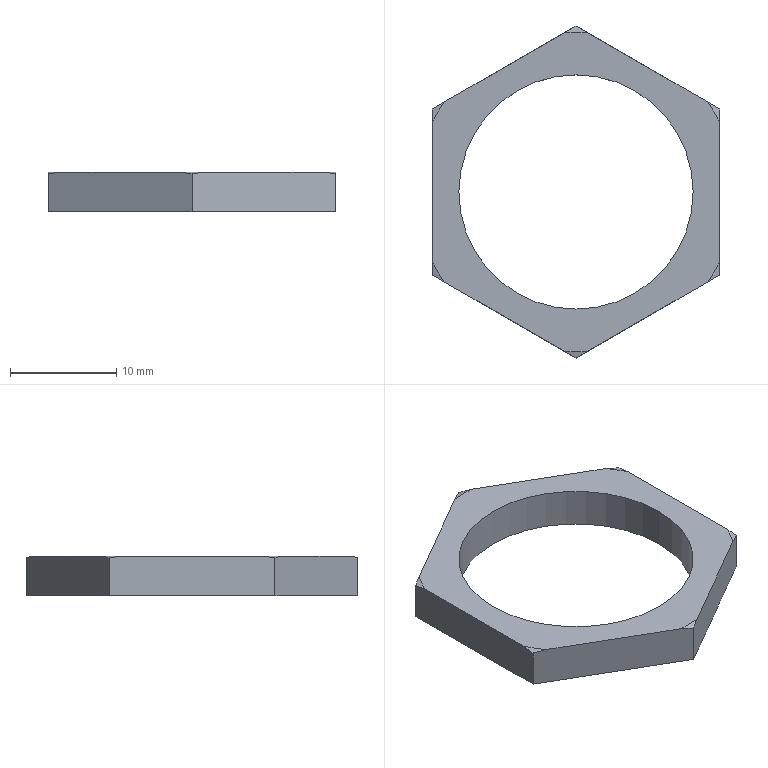Part | STEP file | PN_0023[ PN_0023]_GB/T 808-1988 small hex thin nut M22×1(A3)_Nut M22×1 | 1 solid | 16 faces | box 27 x 31.177 x 3.74 mm | volume 939.292 mm3 | plane 8 | cone 6 | cylinder 2 | commonest cylinder face diameters 22 x2
STEP:
#1=CARTESIAN_POINT('',(-11.,0.,3.74));
#2=VERTEX_POINT('',#1);
#3=CARTESIAN_POINT('',(11.,0.,3.74));
#4=VERTEX_POINT('',#3);
#5=CARTESIAN_POINT('',(0.,0.,3.74));
#6=DIRECTION('',(0.,0.,1.));
#7=DIRECTION('',(1.,0.,0.));
#8=AXIS2_PLACEMENT_3D('',#5,#6,#7);
#9=CIRCLE('',#8,11.);
#10=EDGE_CURVE('',#2,#4,#9,.T.);
#11=ORIENTED_EDGE('',*,*,#10,.T.);
#12=CARTESIAN_POINT('',(11.,0.,0.));
#13=VERTEX_POINT('',#12);
#14=CARTESIAN_POINT('',(11.,0.,3.74));
#15=DIRECTION('',(0.,0.,-1.));
#16=VECTOR('',#15,1000.);
#17=LINE('',#14,#16);
#18=EDGE_CURVE('',#4,#13,#17,.T.);
#19=ORIENTED_EDGE('',*,*,#18,.T.);
#20=CARTESIAN_POINT('',(-11.,0.,0.));
#21=VERTEX_POINT('',#20);
#22=CARTESIAN_POINT('',(0.,0.,0.));
#23=DIRECTION('',(0.,0.,1.));
#24=DIRECTION('',(1.,0.,0.));
#25=AXIS2_PLACEMENT_3D('',#22,#23,#24);
#26=CIRCLE('',#25,11.);
#27=EDGE_CURVE('',#21,#13,#26,.T.);
#28=ORIENTED_EDGE('',*,*,#27,.F.);
#29=CARTESIAN_POINT('',(-11.,0.,3.74));
#30=DIRECTION('',(0.,0.,-1.));
#31=VECTOR('',#30,1000.);
#32=LINE('',#29,#31);
#33=EDGE_CURVE('',#2,#21,#32,.T.);
#34=ORIENTED_EDGE('',*,*,#33,.F.);
#35=EDGE_LOOP('',(#11,#19,#28,#34));
#36=FACE_OUTER_BOUND('',#35,.T.);
#37=CARTESIAN_POINT('',(0.,0.,3.74));
#38=DIRECTION('',(0.,0.,-1.));
#39=DIRECTION('',(-1.,0.,0.));
#40=AXIS2_PLACEMENT_3D('',#37,#38,#39);
#41=CYLINDRICAL_SURFACE('',#40,11.);
#42=ADVANCED_FACE('',(#36),#41,.F.);
#43=ORIENTED_EDGE('',*,*,#10,.F.);
#44=CARTESIAN_POINT('',(0.,0.,3.74));
#45=DIRECTION('',(0.,0.,1.));
#46=DIRECTION('',(1.,0.,0.));
#47=AXIS2_PLACEMENT_3D('',#44,#45,#46);
#48=CIRCLE('',#47,11.);
#49=EDGE_CURVE('',#4,#2,#48,.T.);
#50=ORIENTED_EDGE('',*,*,#49,.F.);
#51=EDGE_LOOP('',(#43,#50));
#52=FACE_BOUND('',#51,.T.);
#53=CARTESIAN_POINT('',(-12.412,8.422,3.74));
#54=VERTEX_POINT('',#53);
#55=CARTESIAN_POINT('',(-13.5,6.538,3.74));
#56=VERTEX_POINT('',#55);
#57=CARTESIAN_POINT('',(0.,0.,3.74));
#58=DIRECTION('',(0.,0.,1.));
#59=DIRECTION('',(1.,0.,0.));
#60=AXIS2_PLACEMENT_3D('',#57,#58,#59);
#61=CIRCLE('',#60,15.);
#62=EDGE_CURVE('',#54,#56,#61,.T.);
#63=ORIENTED_EDGE('',*,*,#62,.T.);
#64=CARTESIAN_POINT('',(-13.5,-6.538,3.74));
#65=VERTEX_POINT('',#64);
#66=CARTESIAN_POINT('',(-13.5,7.794,3.74));
#67=DIRECTION('',(0.,-1.,0.));
#68=VECTOR('',#67,1000.);
#69=LINE('',#66,#68);
#70=EDGE_CURVE('',#56,#65,#69,.T.);
#71=ORIENTED_EDGE('',*,*,#70,.T.);
#72=CARTESIAN_POINT('',(-12.412,-8.422,3.74));
#73=VERTEX_POINT('',#72);
#74=CARTESIAN_POINT('',(0.,0.,3.74));
#75=DIRECTION('',(0.,0.,1.));
#76=DIRECTION('',(1.,0.,0.));
#77=AXIS2_PLACEMENT_3D('',#74,#75,#76);
#78=CIRCLE('',#77,15.);
#79=EDGE_CURVE('',#65,#73,#78,.T.);
#80=ORIENTED_EDGE('',*,*,#79,.T.);
#81=CARTESIAN_POINT('',(-1.088,-14.961,3.74));
#82=VERTEX_POINT('',#81);
#83=CARTESIAN_POINT('',(-13.5,-7.794,3.74));
#84=DIRECTION('',(0.866,-0.5,0.));
#85=VECTOR('',#84,1000.);
#86=LINE('',#83,#85);
#87=EDGE_CURVE('',#73,#82,#86,.T.);
#88=ORIENTED_EDGE('',*,*,#87,.T.);
#89=CARTESIAN_POINT('',(1.088,-14.961,3.74));
#90=VERTEX_POINT('',#89);
#91=CARTESIAN_POINT('',(0.,0.,3.74));
#92=DIRECTION('',(0.,0.,1.));
#93=DIRECTION('',(1.,0.,0.));
#94=AXIS2_PLACEMENT_3D('',#91,#92,#93);
#95=CIRCLE('',#94,15.);
#96=EDGE_CURVE('',#82,#90,#95,.T.);
#97=ORIENTED_EDGE('',*,*,#96,.T.);
#98=CARTESIAN_POINT('',(12.412,-8.422,3.74));
#99=VERTEX_POINT('',#98);
#100=CARTESIAN_POINT('',(0.,-15.588,3.74));
#101=DIRECTION('',(0.866,0.5,0.));
#102=VECTOR('',#101,1000.);
#103=LINE('',#100,#102);
#104=EDGE_CURVE('',#90,#99,#103,.T.);
#105=ORIENTED_EDGE('',*,*,#104,.T.);
#106=CARTESIAN_POINT('',(13.5,-6.538,3.74));
#107=VERTEX_POINT('',#106);
#108=CARTESIAN_POINT('',(0.,0.,3.74));
#109=DIRECTION('',(0.,0.,1.));
#110=DIRECTION('',(1.,0.,0.));
#111=AXIS2_PLACEMENT_3D('',#108,#109,#110);
#112=CIRCLE('',#111,15.);
#113=EDGE_CURVE('',#99,#107,#112,.T.);
#114=ORIENTED_EDGE('',*,*,#113,.T.);
#115=CARTESIAN_POINT('',(13.5,6.538,3.74));
#116=VERTEX_POINT('',#115);
#117=CARTESIAN_POINT('',(13.5,-7.794,3.74));
#118=DIRECTION('',(0.,1.,0.));
#119=VECTOR('',#118,1000.);
#120=LINE('',#117,#119);
#121=EDGE_CURVE('',#107,#116,#120,.T.);
#122=ORIENTED_EDGE('',*,*,#121,.T.);
#123=CARTESIAN_POINT('',(12.412,8.422,3.74));
#124=VERTEX_POINT('',#123);
#125=CARTESIAN_POINT('',(0.,0.,3.74));
#126=DIRECTION('',(0.,0.,1.));
#127=DIRECTION('',(1.,0.,0.));
#128=AXIS2_PLACEMENT_3D('',#125,#126,#127);
#129=CIRCLE('',#128,15.);
#130=EDGE_CURVE('',#116,#124,#129,.T.);
#131=ORIENTED_EDGE('',*,*,#130,.T.);
#132=CARTESIAN_POINT('',(1.088,14.961,3.74));
#133=VERTEX_POINT('',#132);
#134=CARTESIAN_POINT('',(13.5,7.794,3.74));
#135=DIRECTION('',(-0.866,0.5,0.));
#136=VECTOR('',#135,1000.);
#137=LINE('',#134,#136);
#138=EDGE_CURVE('',#124,#133,#137,.T.);
#139=ORIENTED_EDGE('',*,*,#138,.T.);
#140=CARTESIAN_POINT('',(-1.088,14.961,3.74));
#141=VERTEX_POINT('',#140);
#142=CARTESIAN_POINT('',(0.,0.,3.74));
#143=DIRECTION('',(0.,0.,1.));
#144=DIRECTION('',(1.,0.,0.));
#145=AXIS2_PLACEMENT_3D('',#142,#143,#144);
#146=CIRCLE('',#145,15.);
#147=EDGE_CURVE('',#133,#141,#146,.T.);
#148=ORIENTED_EDGE('',*,*,#147,.T.);
#149=CARTESIAN_POINT('',(0.,15.588,3.74));
#150=DIRECTION('',(-0.866,-0.5,0.));
#151=VECTOR('',#150,1000.);
#152=LINE('',#149,#151);
#153=EDGE_CURVE('',#141,#54,#152,.T.);
#154=ORIENTED_EDGE('',*,*,#153,.T.);
#155=EDGE_LOOP('',(#63,#71,#80,#88,#97,#105,#114,#122,#131,#139,#148,#154));
#156=FACE_OUTER_BOUND('',#155,.T.);
#157=CARTESIAN_POINT('',(27.,0.,3.74));
#158=DIRECTION('',(0.,0.,-1.));
#159=DIRECTION('',(-1.,0.,0.));
#160=AXIS2_PLACEMENT_3D('',#157,#158,#159);
#161=PLANE('',#160);
#162=ADVANCED_FACE('',(#52,#156),#161,.F.);
#163=CARTESIAN_POINT('',(13.5,7.794,3.582));
#164=VERTEX_POINT('',#163);
#165=CARTESIAN_POINT('',(13.5,7.794,3.582));
#166=CARTESIAN_POINT('',(13.138,8.003,3.638));
#167=CARTESIAN_POINT('',(12.775,8.213,3.691));
#168=CARTESIAN_POINT('',(12.412,8.422,3.74));
#169=B_SPLINE_CURVE_WITH_KNOTS('',3,(#165,#166,#167,#168),.UNSPECIFIED.,.F.,.F.,(4,4),(0.01126,0.01252),.UNSPECIFIED.);
#170=EDGE_CURVE('',#164,#124,#169,.T.);
#171=ORIENTED_EDGE('',*,*,#170,.F.);
#172=CARTESIAN_POINT('',(13.5,7.794,0.));
#173=VERTEX_POINT('',#172);
#174=CARTESIAN_POINT('',(13.5,7.794,3.74));
#175=DIRECTION('',(0.,0.,-1.));
#176=VECTOR('',#175,1000.);
#177=LINE('',#174,#176);
#178=EDGE_CURVE('',#164,#173,#177,.T.);
#179=ORIENTED_EDGE('',*,*,#178,.T.);
#180=CARTESIAN_POINT('',(0.,15.588,0.));
#181=VERTEX_POINT('',#180);
#182=CARTESIAN_POINT('',(13.5,7.794,0.));
#183=DIRECTION('',(-0.866,0.5,0.));
#184=VECTOR('',#183,1000.);
#185=LINE('',#182,#184);
#186=EDGE_CURVE('',#173,#181,#185,.T.);
#187=ORIENTED_EDGE('',*,*,#186,.T.);
#188=CARTESIAN_POINT('',(0.,15.588,3.582));
#189=VERTEX_POINT('',#188);
#190=CARTESIAN_POINT('',(0.,15.588,3.74));
#191=DIRECTION('',(0.,0.,-1.));
#192=VECTOR('',#191,1000.);
#193=LINE('',#190,#192);
#194=EDGE_CURVE('',#189,#181,#193,.T.);
#195=ORIENTED_EDGE('',*,*,#194,.F.);
#196=CARTESIAN_POINT('',(1.088,14.961,3.74));
#197=CARTESIAN_POINT('',(0.7246,15.17,3.691));
#198=CARTESIAN_POINT('',(0.362,15.379,3.638));
#199=CARTESIAN_POINT('',(0.,15.588,3.582));
#200=B_SPLINE_CURVE_WITH_KNOTS('',3,(#196,#197,#198,#199),.UNSPECIFIED.,.F.,.F.,(4,4),(0.02554,0.02678),.UNSPECIFIED.);
#201=EDGE_CURVE('',#133,#189,#200,.T.);
#202=ORIENTED_EDGE('',*,*,#201,.F.);
#203=ORIENTED_EDGE('',*,*,#138,.F.);
#204=EDGE_LOOP('',(#171,#179,#187,#195,#202,#203));
#205=FACE_OUTER_BOUND('',#204,.T.);
#206=CARTESIAN_POINT('',(13.5,7.794,3.74));
#207=DIRECTION('',(-0.5,-0.866,0.));
#208=DIRECTION('',(0.866,-0.5,0.));
#209=AXIS2_PLACEMENT_3D('',#206,#207,#208);
#210=PLANE('',#209);
#211=ADVANCED_FACE('',(#205),#210,.F.);
#212=CARTESIAN_POINT('',(0.,15.588,3.582));
#213=CARTESIAN_POINT('',(-0.3622,15.379,3.638));
#214=CARTESIAN_POINT('',(-0.7248,15.17,3.691));
#215=CARTESIAN_POINT('',(-1.088,14.961,3.74));
#216=B_SPLINE_CURVE_WITH_KNOTS('',3,(#212,#213,#214,#215),.UNSPECIFIED.,.F.,.F.,(4,4),(0.01126,0.01252),.UNSPECIFIED.);
#217=EDGE_CURVE('',#189,#141,#216,.T.);
#218=ORIENTED_EDGE('',*,*,#217,.F.);
#219=ORIENTED_EDGE('',*,*,#194,.T.);
#220=CARTESIAN_POINT('',(-13.5,7.794,0.));
#221=VERTEX_POINT('',#220);
#222=CARTESIAN_POINT('',(0.,15.588,0.));
#223=DIRECTION('',(-0.866,-0.5,0.));
#224=VECTOR('',#223,1000.);
#225=LINE('',#222,#224);
#226=EDGE_CURVE('',#181,#221,#225,.T.);
#227=ORIENTED_EDGE('',*,*,#226,.T.);
#228=CARTESIAN_POINT('',(-13.5,7.794,3.582));
#229=VERTEX_POINT('',#228);
#230=CARTESIAN_POINT('',(-13.5,7.794,3.74));
#231=DIRECTION('',(0.,0.,-1.));
#232=VECTOR('',#231,1000.);
#233=LINE('',#230,#232);
#234=EDGE_CURVE('',#229,#221,#233,.T.);
#235=ORIENTED_EDGE('',*,*,#234,.F.);
#236=CARTESIAN_POINT('',(-12.412,8.422,3.74));
#237=CARTESIAN_POINT('',(-12.775,8.213,3.691));
#238=CARTESIAN_POINT('',(-13.138,8.003,3.638));
#239=CARTESIAN_POINT('',(-13.5,7.794,3.582));
#240=B_SPLINE_CURVE_WITH_KNOTS('',3,(#236,#237,#238,#239),.UNSPECIFIED.,.F.,.F.,(4,4),(0.02554,0.02678),.UNSPECIFIED.);
#241=EDGE_CURVE('',#54,#229,#240,.T.);
#242=ORIENTED_EDGE('',*,*,#241,.F.);
#243=ORIENTED_EDGE('',*,*,#153,.F.);
#244=EDGE_LOOP('',(#218,#219,#227,#235,#242,#243));
#245=FACE_OUTER_BOUND('',#244,.T.);
#246=CARTESIAN_POINT('',(0.,15.588,3.74));
#247=DIRECTION('',(0.5,-0.866,0.));
#248=DIRECTION('',(0.866,0.5,0.));
#249=AXIS2_PLACEMENT_3D('',#246,#247,#248);
#250=PLANE('',#249);
#251=ADVANCED_FACE('',(#245),#250,.F.);
#252=CARTESIAN_POINT('',(-13.5,7.794,3.582));
#253=CARTESIAN_POINT('',(-13.5,7.376,3.638));
#254=CARTESIAN_POINT('',(-13.5,6.957,3.691));
#255=CARTESIAN_POINT('',(-13.5,6.538,3.74));
#256=B_SPLINE_CURVE_WITH_KNOTS('',3,(#252,#253,#254,#255),.UNSPECIFIED.,.F.,.F.,(4,4),(0.009735,0.011),.UNSPECIFIED.);
#257=EDGE_CURVE('',#229,#56,#256,.T.);
#258=ORIENTED_EDGE('',*,*,#257,.F.);
#259=ORIENTED_EDGE('',*,*,#234,.T.);
#260=CARTESIAN_POINT('',(-13.5,-7.794,0.));
#261=VERTEX_POINT('',#260);
#262=CARTESIAN_POINT('',(-13.5,7.794,0.));
#263=DIRECTION('',(0.,-1.,0.));
#264=VECTOR('',#263,1000.);
#265=LINE('',#262,#264);
#266=EDGE_CURVE('',#221,#261,#265,.T.);
#267=ORIENTED_EDGE('',*,*,#266,.T.);
#268=CARTESIAN_POINT('',(-13.5,-7.794,3.582));
#269=VERTEX_POINT('',#268);
#270=CARTESIAN_POINT('',(-13.5,-7.794,3.74));
#271=DIRECTION('',(0.,0.,-1.));
#272=VECTOR('',#271,1000.);
#273=LINE('',#270,#272);
#274=EDGE_CURVE('',#269,#261,#273,.T.);
#275=ORIENTED_EDGE('',*,*,#274,.F.);
#276=CARTESIAN_POINT('',(-13.5,-6.538,3.74));
#277=CARTESIAN_POINT('',(-13.5,-6.958,3.691));
#278=CARTESIAN_POINT('',(-13.5,-7.376,3.638));
#279=CARTESIAN_POINT('',(-13.5,-7.794,3.582));
#280=B_SPLINE_CURVE_WITH_KNOTS('',3,(#276,#277,#278,#279),.UNSPECIFIED.,.F.,.F.,(4,4),(0.02403,0.02527),.UNSPECIFIED.);
#281=EDGE_CURVE('',#65,#269,#280,.T.);
#282=ORIENTED_EDGE('',*,*,#281,.F.);
#283=ORIENTED_EDGE('',*,*,#70,.F.);
#284=EDGE_LOOP('',(#258,#259,#267,#275,#282,#283));
#285=FACE_OUTER_BOUND('',#284,.T.);
#286=CARTESIAN_POINT('',(-13.5,7.794,3.74));
#287=DIRECTION('',(1.,0.,0.));
#288=DIRECTION('',(0.,1.,0.));
#289=AXIS2_PLACEMENT_3D('',#286,#287,#288);
#290=PLANE('',#289);
#291=ADVANCED_FACE('',(#285),#290,.F.);
#292=CARTESIAN_POINT('',(-13.5,-7.794,3.582));
#293=CARTESIAN_POINT('',(-13.138,-8.003,3.638));
#294=CARTESIAN_POINT('',(-12.775,-8.213,3.691));
#295=CARTESIAN_POINT('',(-12.412,-8.422,3.74));
#296=B_SPLINE_CURVE_WITH_KNOTS('',3,(#292,#293,#294,#295),.UNSPECIFIED.,.F.,.F.,(4,4),(0.01126,0.01252),.UNSPECIFIED.);
#297=EDGE_CURVE('',#269,#73,#296,.T.);
#298=ORIENTED_EDGE('',*,*,#297,.F.);
#299=ORIENTED_EDGE('',*,*,#274,.T.);
#300=CARTESIAN_POINT('',(0.,-15.588,0.));
#301=VERTEX_POINT('',#300);
#302=CARTESIAN_POINT('',(-13.5,-7.794,0.));
#303=DIRECTION('',(0.866,-0.5,0.));
#304=VECTOR('',#303,1000.);
#305=LINE('',#302,#304);
#306=EDGE_CURVE('',#261,#301,#305,.T.);
#307=ORIENTED_EDGE('',*,*,#306,.T.);
#308=CARTESIAN_POINT('',(0.,-15.588,3.582));
#309=VERTEX_POINT('',#308);
#310=CARTESIAN_POINT('',(0.,-15.588,3.74));
#311=DIRECTION('',(0.,0.,-1.));
#312=VECTOR('',#311,1000.);
#313=LINE('',#310,#312);
#314=EDGE_CURVE('',#309,#301,#313,.T.);
#315=ORIENTED_EDGE('',*,*,#314,.F.);
#316=CARTESIAN_POINT('',(-1.088,-14.961,3.74));
#317=CARTESIAN_POINT('',(-0.7246,-15.17,3.691));
#318=CARTESIAN_POINT('',(-0.362,-15.379,3.638));
#319=CARTESIAN_POINT('',(0.,-15.588,3.582));
#320=B_SPLINE_CURVE_WITH_KNOTS('',3,(#316,#317,#318,#319),.UNSPECIFIED.,.F.,.F.,(4,4),(0.02554,0.02678),.UNSPECIFIED.);
#321=EDGE_CURVE('',#82,#309,#320,.T.);
#322=ORIENTED_EDGE('',*,*,#321,.F.);
#323=ORIENTED_EDGE('',*,*,#87,.F.);
#324=EDGE_LOOP('',(#298,#299,#307,#315,#322,#323));
#325=FACE_OUTER_BOUND('',#324,.T.);
#326=CARTESIAN_POINT('',(-13.5,-7.794,3.74));
#327=DIRECTION('',(0.5,0.866,0.));
#328=DIRECTION('',(-0.866,0.5,0.));
#329=AXIS2_PLACEMENT_3D('',#326,#327,#328);
#330=PLANE('',#329);
#331=ADVANCED_FACE('',(#325),#330,.F.);
#332=CARTESIAN_POINT('',(0.,-15.588,3.582));
#333=CARTESIAN_POINT('',(0.3622,-15.379,3.638));
#334=CARTESIAN_POINT('',(0.7248,-15.17,3.691));
#335=CARTESIAN_POINT('',(1.088,-14.961,3.74));
#336=B_SPLINE_CURVE_WITH_KNOTS('',3,(#332,#333,#334,#335),.UNSPECIFIED.,.F.,.F.,(4,4),(0.01126,0.01252),.UNSPECIFIED.);
#337=EDGE_CURVE('',#309,#90,#336,.T.);
#338=ORIENTED_EDGE('',*,*,#337,.F.);
#339=ORIENTED_EDGE('',*,*,#314,.T.);
#340=CARTESIAN_POINT('',(13.5,-7.794,0.));
#341=VERTEX_POINT('',#340);
#342=CARTESIAN_POINT('',(0.,-15.588,0.));
#343=DIRECTION('',(0.866,0.5,0.));
#344=VECTOR('',#343,1000.);
#345=LINE('',#342,#344);
#346=EDGE_CURVE('',#301,#341,#345,.T.);
#347=ORIENTED_EDGE('',*,*,#346,.T.);
#348=CARTESIAN_POINT('',(13.5,-7.794,3.582));
#349=VERTEX_POINT('',#348);
#350=CARTESIAN_POINT('',(13.5,-7.794,3.74));
#351=DIRECTION('',(0.,0.,-1.));
#352=VECTOR('',#351,1000.);
#353=LINE('',#350,#352);
#354=EDGE_CURVE('',#349,#341,#353,.T.);
#355=ORIENTED_EDGE('',*,*,#354,.F.);
#356=CARTESIAN_POINT('',(12.412,-8.422,3.74));
#357=CARTESIAN_POINT('',(12.775,-8.213,3.691));
#358=CARTESIAN_POINT('',(13.138,-8.003,3.638));
#359=CARTESIAN_POINT('',(13.5,-7.794,3.582));
#360=B_SPLINE_CURVE_WITH_KNOTS('',3,(#356,#357,#358,#359),.UNSPECIFIED.,.F.,.F.,(4,4),(0.02554,0.02678),.UNSPECIFIED.);
#361=EDGE_CURVE('',#99,#349,#360,.T.);
#362=ORIENTED_EDGE('',*,*,#361,.F.);
#363=ORIENTED_EDGE('',*,*,#104,.F.);
#364=EDGE_LOOP('',(#338,#339,#347,#355,#362,#363));
#365=FACE_OUTER_BOUND('',#364,.T.);
#366=CARTESIAN_POINT('',(0.,-15.588,3.74));
#367=DIRECTION('',(-0.5,0.866,0.));
#368=DIRECTION('',(-0.866,-0.5,0.));
#369=AXIS2_PLACEMENT_3D('',#366,#367,#368);
#370=PLANE('',#369);
#371=ADVANCED_FACE('',(#365),#370,.F.);
#372=CARTESIAN_POINT('',(13.5,-7.794,3.582));
#373=CARTESIAN_POINT('',(13.5,-7.376,3.638));
#374=CARTESIAN_POINT('',(13.5,-6.957,3.691));
#375=CARTESIAN_POINT('',(13.5,-6.538,3.74));
#376=B_SPLINE_CURVE_WITH_KNOTS('',3,(#372,#373,#374,#375),.UNSPECIFIED.,.F.,.F.,(4,4),(0.009735,0.011),.UNSPECIFIED.);
#377=EDGE_CURVE('',#349,#107,#376,.T.);
#378=ORIENTED_EDGE('',*,*,#377,.F.);
#379=ORIENTED_EDGE('',*,*,#354,.T.);
#380=CARTESIAN_POINT('',(13.5,-7.794,0.));
#381=DIRECTION('',(0.,1.,0.));
#382=VECTOR('',#381,1000.);
#383=LINE('',#380,#382);
#384=EDGE_CURVE('',#341,#173,#383,.T.);
#385=ORIENTED_EDGE('',*,*,#384,.T.);
#386=ORIENTED_EDGE('',*,*,#178,.F.);
#387=CARTESIAN_POINT('',(13.5,6.538,3.74));
#388=CARTESIAN_POINT('',(13.5,6.958,3.691));
#389=CARTESIAN_POINT('',(13.5,7.376,3.638));
#390=CARTESIAN_POINT('',(13.5,7.794,3.582));
#391=B_SPLINE_CURVE_WITH_KNOTS('',3,(#387,#388,#389,#390),.UNSPECIFIED.,.F.,.F.,(4,4),(0.02403,0.02527),.UNSPECIFIED.);
#392=EDGE_CURVE('',#116,#164,#391,.T.);
#393=ORIENTED_EDGE('',*,*,#392,.F.);
#394=ORIENTED_EDGE('',*,*,#121,.F.);
#395=EDGE_LOOP('',(#378,#379,#385,#386,#393,#394));
#396=FACE_OUTER_BOUND('',#395,.T.);
#397=CARTESIAN_POINT('',(13.5,-7.794,3.74));
#398=DIRECTION('',(-1.,0.,0.));
#399=DIRECTION('',(0.,-1.,0.));
#400=AXIS2_PLACEMENT_3D('',#397,#398,#399);
#401=PLANE('',#400);
#402=ADVANCED_FACE('',(#396),#401,.F.);
#403=ORIENTED_EDGE('',*,*,#186,.F.);
#404=ORIENTED_EDGE('',*,*,#384,.F.);
#405=ORIENTED_EDGE('',*,*,#346,.F.);
#406=ORIENTED_EDGE('',*,*,#306,.F.);
#407=ORIENTED_EDGE('',*,*,#266,.F.);
#408=ORIENTED_EDGE('',*,*,#226,.F.);
#409=EDGE_LOOP('',(#403,#404,#405,#406,#407,#408));
#410=FACE_OUTER_BOUND('',#409,.T.);
#411=ORIENTED_EDGE('',*,*,#27,.T.);
#412=CARTESIAN_POINT('',(0.,0.,0.));
#413=DIRECTION('',(0.,0.,1.));
#414=DIRECTION('',(1.,0.,0.));
#415=AXIS2_PLACEMENT_3D('',#412,#413,#414);
#416=CIRCLE('',#415,11.);
#417=EDGE_CURVE('',#13,#21,#416,.T.);
#418=ORIENTED_EDGE('',*,*,#417,.T.);
#419=EDGE_LOOP('',(#411,#418));
#420=FACE_BOUND('',#419,.T.);
#421=CARTESIAN_POINT('',(27.,0.,0.));
#422=DIRECTION('',(0.,0.,-1.));
#423=DIRECTION('',(-1.,0.,0.));
#424=AXIS2_PLACEMENT_3D('',#421,#422,#423);
#425=PLANE('',#424);
#426=ADVANCED_FACE('',(#410,#420),#425,.T.);
#427=ORIENTED_EDGE('',*,*,#18,.F.);
#428=ORIENTED_EDGE('',*,*,#49,.T.);
#429=ORIENTED_EDGE('',*,*,#33,.T.);
#430=ORIENTED_EDGE('',*,*,#417,.F.);
#431=EDGE_LOOP('',(#427,#428,#429,#430));
#432=FACE_OUTER_BOUND('',#431,.T.);
#433=CARTESIAN_POINT('',(0.,0.,3.74));
#434=DIRECTION('',(0.,0.,-1.));
#435=DIRECTION('',(-1.,0.,0.));
#436=AXIS2_PLACEMENT_3D('',#433,#434,#435);
#437=CYLINDRICAL_SURFACE('',#436,11.);
#438=ADVANCED_FACE('',(#432),#437,.F.);
#439=ORIENTED_EDGE('',*,*,#170,.T.);
#440=ORIENTED_EDGE('',*,*,#130,.F.);
#441=ORIENTED_EDGE('',*,*,#392,.T.);
#442=EDGE_LOOP('',(#439,#440,#441));
#443=FACE_OUTER_BOUND('',#442,.T.);
#444=CARTESIAN_POINT('',(0.,0.,3.74));
#445=DIRECTION('',(0.,0.,-1.));
#446=DIRECTION('',(1.,0.,0.));
#447=AXIS2_PLACEMENT_3D('',#444,#445,#446);
#448=CONICAL_SURFACE('',#447,15.,1.309);
#449=ADVANCED_FACE('',(#443),#448,.T.);
#450=ORIENTED_EDGE('',*,*,#361,.T.);
#451=ORIENTED_EDGE('',*,*,#377,.T.);
#452=ORIENTED_EDGE('',*,*,#113,.F.);
#453=EDGE_LOOP('',(#450,#451,#452));
#454=FACE_OUTER_BOUND('',#453,.T.);
#455=CARTESIAN_POINT('',(0.,0.,3.74));
#456=DIRECTION('',(0.,0.,-1.));
#457=DIRECTION('',(1.,0.,0.));
#458=AXIS2_PLACEMENT_3D('',#455,#456,#457);
#459=CONICAL_SURFACE('',#458,15.,1.309);
#460=ADVANCED_FACE('',(#454),#459,.T.);
#461=ORIENTED_EDGE('',*,*,#321,.T.);
#462=ORIENTED_EDGE('',*,*,#337,.T.);
#463=ORIENTED_EDGE('',*,*,#96,.F.);
#464=EDGE_LOOP('',(#461,#462,#463));
#465=FACE_OUTER_BOUND('',#464,.T.);
#466=CARTESIAN_POINT('',(0.,0.,3.74));
#467=DIRECTION('',(0.,0.,-1.));
#468=DIRECTION('',(1.,0.,0.));
#469=AXIS2_PLACEMENT_3D('',#466,#467,#468);
#470=CONICAL_SURFACE('',#469,15.,1.309);
#471=ADVANCED_FACE('',(#465),#470,.T.);
#472=ORIENTED_EDGE('',*,*,#281,.T.);
#473=ORIENTED_EDGE('',*,*,#297,.T.);
#474=ORIENTED_EDGE('',*,*,#79,.F.);
#475=EDGE_LOOP('',(#472,#473,#474));
#476=FACE_OUTER_BOUND('',#475,.T.);
#477=CARTESIAN_POINT('',(0.,0.,3.74));
#478=DIRECTION('',(0.,0.,-1.));
#479=DIRECTION('',(1.,0.,0.));
#480=AXIS2_PLACEMENT_3D('',#477,#478,#479);
#481=CONICAL_SURFACE('',#480,15.,1.309);
#482=ADVANCED_FACE('',(#476),#481,.T.);
#483=ORIENTED_EDGE('',*,*,#241,.T.);
#484=ORIENTED_EDGE('',*,*,#257,.T.);
#485=ORIENTED_EDGE('',*,*,#62,.F.);
#486=EDGE_LOOP('',(#483,#484,#485));
#487=FACE_OUTER_BOUND('',#486,.T.);
#488=CARTESIAN_POINT('',(0.,0.,3.74));
#489=DIRECTION('',(0.,0.,-1.));
#490=DIRECTION('',(1.,0.,0.));
#491=AXIS2_PLACEMENT_3D('',#488,#489,#490);
#492=CONICAL_SURFACE('',#491,15.,1.309);
#493=ADVANCED_FACE('',(#487),#492,.T.);
#494=ORIENTED_EDGE('',*,*,#201,.T.);
#495=ORIENTED_EDGE('',*,*,#217,.T.);
#496=ORIENTED_EDGE('',*,*,#147,.F.);
#497=EDGE_LOOP('',(#494,#495,#496));
#498=FACE_OUTER_BOUND('',#497,.T.);
#499=CARTESIAN_POINT('',(0.,0.,3.74));
#500=DIRECTION('',(0.,0.,-1.));
#501=DIRECTION('',(1.,0.,0.));
#502=AXIS2_PLACEMENT_3D('',#499,#500,#501);
#503=CONICAL_SURFACE('',#502,15.,1.309);
#504=ADVANCED_FACE('',(#498),#503,.T.);
#505=CLOSED_SHELL('',(#42,#162,#211,#251,#291,#331,#371,#402,#426,#438,#449,#460,#471,#482,#493,#504));
#506=MANIFOLD_SOLID_BREP('',#505);
#507=CARTESIAN_POINT('',(0.,0.,0.));
#508=DIRECTION('',(0.,0.,1.));
#509=DIRECTION('',(1.,0.,0.));
#510=AXIS2_PLACEMENT_3D('',#507,#508,#509);
#511=(LENGTH_UNIT()NAMED_UNIT(*)SI_UNIT(.MILLI.,.METRE.));
#512=UNCERTAINTY_MEASURE_WITH_UNIT(LENGTH_MEASURE(0.00001),#511,'','');
#513=(NAMED_UNIT(*)PLANE_ANGLE_UNIT()SI_UNIT($,.RADIAN.));
#514=(NAMED_UNIT(*)SI_UNIT($,.STERADIAN.)SOLID_ANGLE_UNIT());
#515=(GEOMETRIC_REPRESENTATION_CONTEXT(3)GLOBAL_UNCERTAINTY_ASSIGNED_CONTEXT((#512))GLOBAL_UNIT_ASSIGNED_CONTEXT((#511,#513,#514))REPRESENTATION_CONTEXT('',''));
#516=ADVANCED_BREP_SHAPE_REPRESENTATION('',(#506,#510),#515);